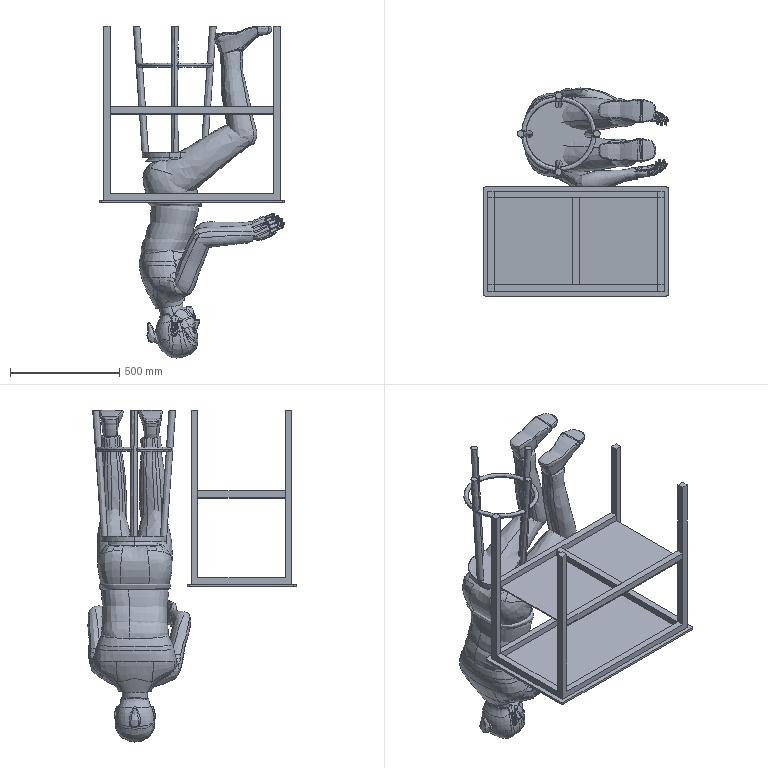Part | SolidWorks | 5 solids | 806 faces | box 851.002 x 954.449 x 1522 mm | volume 114343551 mm3 | spline 733 | plane 66 | cylinder 7 | commonest cylinder face diameters 20 x4 300 x3